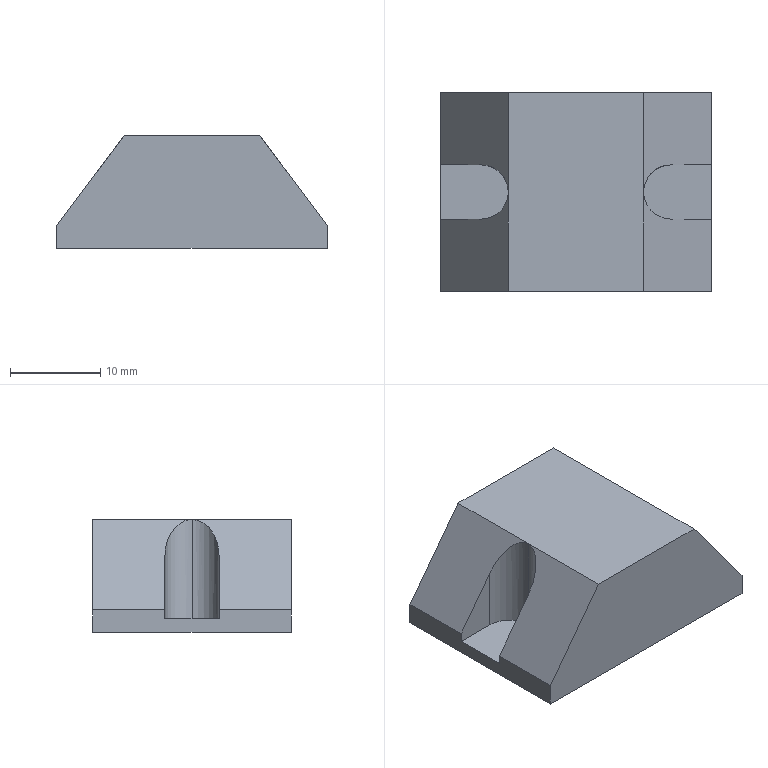Part | STEP file | Wire clamp block | 1 solid | 17 faces | box 30 x 22 x 12.5 mm | volume 6136 mm3 | plane 14 | cylinder 3 | commonest cylinder face diameters 6 x3
STEP:
#1=CARTESIAN_POINT('',(-7.5,0.,1.5));
#2=VERTEX_POINT('',#1);
#3=CARTESIAN_POINT('',(-10.5,3.,1.5));
#4=VERTEX_POINT('',#3);
#5=CARTESIAN_POINT('',(-10.5,0.,1.5));
#6=DIRECTION('',(0.,0.,1.));
#7=DIRECTION('',(1.,0.,0.));
#8=AXIS2_PLACEMENT_3D('',#5,#6,#7);
#9=CIRCLE('',#8,3.);
#10=EDGE_CURVE('',#2,#4,#9,.T.);
#11=ORIENTED_EDGE('',*,*,#10,.F.);
#12=CARTESIAN_POINT('',(-7.5,0.,12.486));
#13=VERTEX_POINT('',#12);
#14=CARTESIAN_POINT('',(-7.5,0.,1.5));
#15=DIRECTION('',(0.,0.,1.));
#16=VECTOR('',#15,1000.);
#17=LINE('',#14,#16);
#18=EDGE_CURVE('',#2,#13,#17,.T.);
#19=ORIENTED_EDGE('',*,*,#18,.T.);
#20=CARTESIAN_POINT('',(-10.5,3.,8.491));
#21=VERTEX_POINT('',#20);
#22=CARTESIAN_POINT('',(-7.5,0.,12.486));
#23=CARTESIAN_POINT('',(-7.5,1.757,12.486));
#24=CARTESIAN_POINT('',(-8.743,3.,10.831));
#25=CARTESIAN_POINT('',(-10.5,3.,8.491));
#26=(BOUNDED_CURVE()B_SPLINE_CURVE(3,(#22,#23,#24,#25),.UNSPECIFIED.,.F.,.T.)B_SPLINE_CURVE_WITH_KNOTS((4,4),(0.,1.571),.UNSPECIFIED.)CURVE()GEOMETRIC_REPRESENTATION_ITEM()RATIONAL_B_SPLINE_CURVE((1.,0.8047,0.8047,1.))REPRESENTATION_ITEM(''));
#27=EDGE_CURVE('',#13,#21,#26,.T.);
#28=ORIENTED_EDGE('',*,*,#27,.T.);
#29=CARTESIAN_POINT('',(-10.5,3.,1.5));
#30=DIRECTION('',(0.,0.,1.));
#31=VECTOR('',#30,1000.);
#32=LINE('',#29,#31);
#33=EDGE_CURVE('',#4,#21,#32,.T.);
#34=ORIENTED_EDGE('',*,*,#33,.F.);
#35=EDGE_LOOP('',(#11,#19,#28,#34));
#36=FACE_OUTER_BOUND('',#35,.T.);
#37=CARTESIAN_POINT('',(-10.5,0.,1.5));
#38=DIRECTION('',(0.,0.,1.));
#39=DIRECTION('',(1.,0.,0.));
#40=AXIS2_PLACEMENT_3D('',#37,#38,#39);
#41=CYLINDRICAL_SURFACE('',#40,3.);
#42=ADVANCED_FACE('',(#36),#41,.F.);
#43=CARTESIAN_POINT('',(-15.,-11.,0.));
#44=VERTEX_POINT('',#43);
#45=CARTESIAN_POINT('',(-15.,11.,0.));
#46=VERTEX_POINT('',#45);
#47=CARTESIAN_POINT('',(-15.,11.,0.));
#48=DIRECTION('',(0.,1.,0.));
#49=VECTOR('',#48,1000.);
#50=LINE('',#47,#49);
#51=EDGE_CURVE('',#44,#46,#50,.T.);
#52=ORIENTED_EDGE('',*,*,#51,.T.);
#53=CARTESIAN_POINT('',(15.,11.,0.));
#54=VERTEX_POINT('',#53);
#55=CARTESIAN_POINT('',(15.,11.,0.));
#56=DIRECTION('',(1.,0.,0.));
#57=VECTOR('',#56,1000.);
#58=LINE('',#55,#57);
#59=EDGE_CURVE('',#46,#54,#58,.T.);
#60=ORIENTED_EDGE('',*,*,#59,.T.);
#61=CARTESIAN_POINT('',(15.,-11.,0.));
#62=VERTEX_POINT('',#61);
#63=CARTESIAN_POINT('',(15.,11.,0.));
#64=DIRECTION('',(0.,-1.,0.));
#65=VECTOR('',#64,1000.);
#66=LINE('',#63,#65);
#67=EDGE_CURVE('',#54,#62,#66,.T.);
#68=ORIENTED_EDGE('',*,*,#67,.T.);
#69=CARTESIAN_POINT('',(15.,-11.,0.));
#70=DIRECTION('',(-1.,0.,0.));
#71=VECTOR('',#70,1000.);
#72=LINE('',#69,#71);
#73=EDGE_CURVE('',#62,#44,#72,.T.);
#74=ORIENTED_EDGE('',*,*,#73,.T.);
#75=EDGE_LOOP('',(#52,#60,#68,#74));
#76=FACE_OUTER_BOUND('',#75,.T.);
#77=CARTESIAN_POINT('',(15.,11.,0.));
#78=DIRECTION('',(0.,0.,-1.));
#79=DIRECTION('',(-1.,0.,0.));
#80=AXIS2_PLACEMENT_3D('',#77,#78,#79);
#81=PLANE('',#80);
#82=ADVANCED_FACE('',(#76),#81,.T.);
#83=CARTESIAN_POINT('',(-7.489,11.,12.5));
#84=VERTEX_POINT('',#83);
#85=CARTESIAN_POINT('',(-15.,11.,2.5));
#86=VERTEX_POINT('',#85);
#87=CARTESIAN_POINT('',(-7.489,11.,12.5));
#88=DIRECTION('',(-0.6006,0.,-0.7996));
#89=VECTOR('',#88,1000.);
#90=LINE('',#87,#89);
#91=EDGE_CURVE('',#84,#86,#90,.T.);
#92=ORIENTED_EDGE('',*,*,#91,.F.);
#93=CARTESIAN_POINT('',(7.489,11.,12.5));
#94=VERTEX_POINT('',#93);
#95=CARTESIAN_POINT('',(-15.,11.,12.5));
#96=DIRECTION('',(-1.,0.,0.));
#97=VECTOR('',#96,1000.);
#98=LINE('',#95,#97);
#99=EDGE_CURVE('',#94,#84,#98,.T.);
#100=ORIENTED_EDGE('',*,*,#99,.F.);
#101=CARTESIAN_POINT('',(15.,11.,2.5));
#102=VERTEX_POINT('',#101);
#103=CARTESIAN_POINT('',(15.,11.,2.5));
#104=DIRECTION('',(-0.6006,0.,0.7996));
#105=VECTOR('',#104,1000.);
#106=LINE('',#103,#105);
#107=EDGE_CURVE('',#102,#94,#106,.T.);
#108=ORIENTED_EDGE('',*,*,#107,.F.);
#109=CARTESIAN_POINT('',(15.,11.,12.5));
#110=DIRECTION('',(0.,0.,1.));
#111=VECTOR('',#110,1000.);
#112=LINE('',#109,#111);
#113=EDGE_CURVE('',#54,#102,#112,.T.);
#114=ORIENTED_EDGE('',*,*,#113,.F.);
#115=ORIENTED_EDGE('',*,*,#59,.F.);
#116=CARTESIAN_POINT('',(-15.,11.,12.5));
#117=DIRECTION('',(0.,0.,-1.));
#118=VECTOR('',#117,1000.);
#119=LINE('',#116,#118);
#120=EDGE_CURVE('',#86,#46,#119,.T.);
#121=ORIENTED_EDGE('',*,*,#120,.F.);
#122=EDGE_LOOP('',(#92,#100,#108,#114,#115,#121));
#123=FACE_OUTER_BOUND('',#122,.T.);
#124=CARTESIAN_POINT('',(-15.,11.,12.5));
#125=DIRECTION('',(0.,-1.,0.));
#126=DIRECTION('',(0.,0.,-1.));
#127=AXIS2_PLACEMENT_3D('',#124,#125,#126);
#128=PLANE('',#127);
#129=ADVANCED_FACE('',(#123),#128,.F.);
#130=CARTESIAN_POINT('',(-15.,-3.,2.5));
#131=VERTEX_POINT('',#130);
#132=CARTESIAN_POINT('',(-15.,-3.,1.5));
#133=VERTEX_POINT('',#132);
#134=CARTESIAN_POINT('',(-15.,-3.,1.5));
#135=DIRECTION('',(0.,0.,-1.));
#136=VECTOR('',#135,1000.);
#137=LINE('',#134,#136);
#138=EDGE_CURVE('',#131,#133,#137,.T.);
#139=ORIENTED_EDGE('',*,*,#138,.T.);
#140=CARTESIAN_POINT('',(-15.,3.,1.5));
#141=VERTEX_POINT('',#140);
#142=CARTESIAN_POINT('',(-15.,-11.,1.5));
#143=DIRECTION('',(0.,-1.,0.));
#144=VECTOR('',#143,1000.);
#145=LINE('',#142,#144);
#146=EDGE_CURVE('',#141,#133,#145,.T.);
#147=ORIENTED_EDGE('',*,*,#146,.F.);
#148=CARTESIAN_POINT('',(-15.,3.,2.5));
#149=VERTEX_POINT('',#148);
#150=CARTESIAN_POINT('',(-15.,3.,1.5));
#151=DIRECTION('',(0.,0.,1.));
#152=VECTOR('',#151,1000.);
#153=LINE('',#150,#152);
#154=EDGE_CURVE('',#141,#149,#153,.T.);
#155=ORIENTED_EDGE('',*,*,#154,.T.);
#156=CARTESIAN_POINT('',(-15.,-11.,2.5));
#157=DIRECTION('',(0.,-1.,0.));
#158=VECTOR('',#157,1000.);
#159=LINE('',#156,#158);
#160=EDGE_CURVE('',#86,#149,#159,.T.);
#161=ORIENTED_EDGE('',*,*,#160,.F.);
#162=ORIENTED_EDGE('',*,*,#120,.T.);
#163=ORIENTED_EDGE('',*,*,#51,.F.);
#164=CARTESIAN_POINT('',(-15.,-11.,2.5));
#165=VERTEX_POINT('',#164);
#166=CARTESIAN_POINT('',(-15.,-11.,12.5));
#167=DIRECTION('',(0.,0.,-1.));
#168=VECTOR('',#167,1000.);
#169=LINE('',#166,#168);
#170=EDGE_CURVE('',#165,#44,#169,.T.);
#171=ORIENTED_EDGE('',*,*,#170,.F.);
#172=CARTESIAN_POINT('',(-15.,-11.,2.5));
#173=DIRECTION('',(0.,-1.,0.));
#174=VECTOR('',#173,1000.);
#175=LINE('',#172,#174);
#176=EDGE_CURVE('',#131,#165,#175,.T.);
#177=ORIENTED_EDGE('',*,*,#176,.F.);
#178=EDGE_LOOP('',(#139,#147,#155,#161,#162,#163,#171,#177));
#179=FACE_OUTER_BOUND('',#178,.T.);
#180=CARTESIAN_POINT('',(-15.,-11.,12.5));
#181=DIRECTION('',(1.,0.,0.));
#182=DIRECTION('',(0.,0.,-1.));
#183=AXIS2_PLACEMENT_3D('',#180,#181,#182);
#184=PLANE('',#183);
#185=ADVANCED_FACE('',(#179),#184,.F.);
#186=CARTESIAN_POINT('',(-7.489,-11.,12.5));
#187=VERTEX_POINT('',#186);
#188=CARTESIAN_POINT('',(-15.,-11.,2.5));
#189=DIRECTION('',(0.6006,0.,0.7996));
#190=VECTOR('',#189,1000.);
#191=LINE('',#188,#190);
#192=EDGE_CURVE('',#165,#187,#191,.T.);
#193=ORIENTED_EDGE('',*,*,#192,.F.);
#194=ORIENTED_EDGE('',*,*,#170,.T.);
#195=ORIENTED_EDGE('',*,*,#73,.F.);
#196=CARTESIAN_POINT('',(15.,-11.,2.5));
#197=VERTEX_POINT('',#196);
#198=CARTESIAN_POINT('',(15.,-11.,12.5));
#199=DIRECTION('',(0.,0.,-1.));
#200=VECTOR('',#199,1000.);
#201=LINE('',#198,#200);
#202=EDGE_CURVE('',#197,#62,#201,.T.);
#203=ORIENTED_EDGE('',*,*,#202,.F.);
#204=CARTESIAN_POINT('',(7.489,-11.,12.5));
#205=VERTEX_POINT('',#204);
#206=CARTESIAN_POINT('',(7.489,-11.,12.5));
#207=DIRECTION('',(0.6006,0.,-0.7996));
#208=VECTOR('',#207,1000.);
#209=LINE('',#206,#208);
#210=EDGE_CURVE('',#205,#197,#209,.T.);
#211=ORIENTED_EDGE('',*,*,#210,.F.);
#212=CARTESIAN_POINT('',(-15.,-11.,12.5));
#213=DIRECTION('',(1.,0.,0.));
#214=VECTOR('',#213,1000.);
#215=LINE('',#212,#214);
#216=EDGE_CURVE('',#187,#205,#215,.T.);
#217=ORIENTED_EDGE('',*,*,#216,.F.);
#218=EDGE_LOOP('',(#193,#194,#195,#203,#211,#217));
#219=FACE_OUTER_BOUND('',#218,.T.);
#220=CARTESIAN_POINT('',(-15.,-11.,12.5));
#221=DIRECTION('',(0.,1.,0.));
#222=DIRECTION('',(0.,0.,1.));
#223=AXIS2_PLACEMENT_3D('',#220,#221,#222);
#224=PLANE('',#223);
#225=ADVANCED_FACE('',(#219),#224,.F.);
#226=CARTESIAN_POINT('',(15.,3.,2.5));
#227=VERTEX_POINT('',#226);
#228=CARTESIAN_POINT('',(15.,3.,1.5));
#229=VERTEX_POINT('',#228);
#230=CARTESIAN_POINT('',(15.,3.,1.5));
#231=DIRECTION('',(0.,0.,-1.));
#232=VECTOR('',#231,1000.);
#233=LINE('',#230,#232);
#234=EDGE_CURVE('',#227,#229,#233,.T.);
#235=ORIENTED_EDGE('',*,*,#234,.T.);
#236=CARTESIAN_POINT('',(15.,-3.,1.5));
#237=VERTEX_POINT('',#236);
#238=CARTESIAN_POINT('',(15.,-11.,1.5));
#239=DIRECTION('',(0.,1.,0.));
#240=VECTOR('',#239,1000.);
#241=LINE('',#238,#240);
#242=EDGE_CURVE('',#237,#229,#241,.T.);
#243=ORIENTED_EDGE('',*,*,#242,.F.);
#244=CARTESIAN_POINT('',(15.,-3.,2.5));
#245=VERTEX_POINT('',#244);
#246=CARTESIAN_POINT('',(15.,-3.,1.5));
#247=DIRECTION('',(0.,0.,1.));
#248=VECTOR('',#247,1000.);
#249=LINE('',#246,#248);
#250=EDGE_CURVE('',#237,#245,#249,.T.);
#251=ORIENTED_EDGE('',*,*,#250,.T.);
#252=CARTESIAN_POINT('',(15.,-11.,2.5));
#253=DIRECTION('',(0.,1.,0.));
#254=VECTOR('',#253,1000.);
#255=LINE('',#252,#254);
#256=EDGE_CURVE('',#197,#245,#255,.T.);
#257=ORIENTED_EDGE('',*,*,#256,.F.);
#258=ORIENTED_EDGE('',*,*,#202,.T.);
#259=ORIENTED_EDGE('',*,*,#67,.F.);
#260=ORIENTED_EDGE('',*,*,#113,.T.);
#261=CARTESIAN_POINT('',(15.,-11.,2.5));
#262=DIRECTION('',(0.,1.,0.));
#263=VECTOR('',#262,1000.);
#264=LINE('',#261,#263);
#265=EDGE_CURVE('',#227,#102,#264,.T.);
#266=ORIENTED_EDGE('',*,*,#265,.F.);
#267=EDGE_LOOP('',(#235,#243,#251,#257,#258,#259,#260,#266));
#268=FACE_OUTER_BOUND('',#267,.T.);
#269=CARTESIAN_POINT('',(15.,-11.,12.5));
#270=DIRECTION('',(-1.,0.,0.));
#271=DIRECTION('',(0.,0.,1.));
#272=AXIS2_PLACEMENT_3D('',#269,#270,#271);
#273=PLANE('',#272);
#274=ADVANCED_FACE('',(#268),#273,.F.);
#275=CARTESIAN_POINT('',(-10.5,-3.,8.491));
#276=VERTEX_POINT('',#275);
#277=CARTESIAN_POINT('',(-10.5,-3.,8.491));
#278=CARTESIAN_POINT('',(-8.743,-3.,10.831));
#279=CARTESIAN_POINT('',(-7.5,-1.757,12.486));
#280=CARTESIAN_POINT('',(-7.5,0.,12.486));
#281=(BOUNDED_CURVE()B_SPLINE_CURVE(3,(#277,#278,#279,#280),.UNSPECIFIED.,.F.,.F.)B_SPLINE_CURVE_WITH_KNOTS((4,4),(4.712,6.283),.UNSPECIFIED.)CURVE()GEOMETRIC_REPRESENTATION_ITEM()RATIONAL_B_SPLINE_CURVE((1.,0.8047,0.8047,1.))REPRESENTATION_ITEM(''));
#282=EDGE_CURVE('',#276,#13,#281,.T.);
#283=ORIENTED_EDGE('',*,*,#282,.F.);
#284=CARTESIAN_POINT('',(-15.,-3.,2.5));
#285=DIRECTION('',(0.6006,0.,0.7996));
#286=VECTOR('',#285,1000.);
#287=LINE('',#284,#286);
#288=EDGE_CURVE('',#131,#276,#287,.T.);
#289=ORIENTED_EDGE('',*,*,#288,.F.);
#290=ORIENTED_EDGE('',*,*,#176,.T.);
#291=ORIENTED_EDGE('',*,*,#192,.T.);
#292=CARTESIAN_POINT('',(-7.489,19.,12.5));
#293=DIRECTION('',(0.,-1.,0.));
#294=VECTOR('',#293,1000.);
#295=LINE('',#292,#294);
#296=EDGE_CURVE('',#84,#187,#295,.T.);
#297=ORIENTED_EDGE('',*,*,#296,.F.);
#298=ORIENTED_EDGE('',*,*,#91,.T.);
#299=ORIENTED_EDGE('',*,*,#160,.T.);
#300=CARTESIAN_POINT('',(-15.,3.,2.5));
#301=DIRECTION('',(-0.6006,0.,-0.7996));
#302=VECTOR('',#301,1000.);
#303=LINE('',#300,#302);
#304=EDGE_CURVE('',#21,#149,#303,.T.);
#305=ORIENTED_EDGE('',*,*,#304,.F.);
#306=ORIENTED_EDGE('',*,*,#27,.F.);
#307=EDGE_LOOP('',(#283,#289,#290,#291,#297,#298,#299,#305,#306));
#308=FACE_OUTER_BOUND('',#307,.T.);
#309=CARTESIAN_POINT('',(-15.,19.,2.5));
#310=DIRECTION('',(0.7996,0.,-0.6006));
#311=DIRECTION('',(-0.6006,0.,-0.7996));
#312=AXIS2_PLACEMENT_3D('',#309,#310,#311);
#313=PLANE('',#312);
#314=ADVANCED_FACE('',(#308),#313,.F.);
#315=ORIENTED_EDGE('',*,*,#296,.T.);
#316=ORIENTED_EDGE('',*,*,#216,.T.);
#317=CARTESIAN_POINT('',(7.489,11.,12.5));
#318=DIRECTION('',(0.,-1.,0.));
#319=VECTOR('',#318,1000.);
#320=LINE('',#317,#319);
#321=EDGE_CURVE('',#94,#205,#320,.T.);
#322=ORIENTED_EDGE('',*,*,#321,.F.);
#323=ORIENTED_EDGE('',*,*,#99,.T.);
#324=EDGE_LOOP('',(#315,#316,#322,#323));
#325=FACE_OUTER_BOUND('',#324,.T.);
#326=CARTESIAN_POINT('',(15.,11.,12.5));
#327=DIRECTION('',(0.,0.,-1.));
#328=DIRECTION('',(-1.,0.,0.));
#329=AXIS2_PLACEMENT_3D('',#326,#327,#328);
#330=PLANE('',#329);
#331=ADVANCED_FACE('',(#325),#330,.F.);
#332=CARTESIAN_POINT('',(10.5,3.,8.491));
#333=VERTEX_POINT('',#332);
#334=CARTESIAN_POINT('',(15.,3.,2.5));
#335=DIRECTION('',(-0.6006,0.,0.7996));
#336=VECTOR('',#335,1000.);
#337=LINE('',#334,#336);
#338=EDGE_CURVE('',#227,#333,#337,.T.);
#339=ORIENTED_EDGE('',*,*,#338,.F.);
#340=ORIENTED_EDGE('',*,*,#265,.T.);
#341=ORIENTED_EDGE('',*,*,#107,.T.);
#342=ORIENTED_EDGE('',*,*,#321,.T.);
#343=ORIENTED_EDGE('',*,*,#210,.T.);
#344=ORIENTED_EDGE('',*,*,#256,.T.);
#345=CARTESIAN_POINT('',(10.5,-3.,8.491));
#346=VERTEX_POINT('',#345);
#347=CARTESIAN_POINT('',(15.,-3.,2.5));
#348=DIRECTION('',(0.6006,0.,-0.7996));
#349=VECTOR('',#348,1000.);
#350=LINE('',#347,#349);
#351=EDGE_CURVE('',#346,#245,#350,.T.);
#352=ORIENTED_EDGE('',*,*,#351,.F.);
#353=CARTESIAN_POINT('',(10.5,3.,8.491));
#354=CARTESIAN_POINT('',(4.5,3.,16.48));
#355=CARTESIAN_POINT('',(4.5,-3.,16.48));
#356=CARTESIAN_POINT('',(10.5,-3.,8.491));
#357=(BOUNDED_CURVE()B_SPLINE_CURVE(3,(#353,#354,#355,#356),.UNSPECIFIED.,.F.,.F.)B_SPLINE_CURVE_WITH_KNOTS((4,4),(4.712,7.854),.UNSPECIFIED.)CURVE()GEOMETRIC_REPRESENTATION_ITEM()RATIONAL_B_SPLINE_CURVE((1.,0.3333,0.3333,1.))REPRESENTATION_ITEM(''));
#358=EDGE_CURVE('',#333,#346,#357,.T.);
#359=ORIENTED_EDGE('',*,*,#358,.F.);
#360=EDGE_LOOP('',(#339,#340,#341,#342,#343,#344,#352,#359));
#361=FACE_OUTER_BOUND('',#360,.T.);
#362=CARTESIAN_POINT('',(15.,19.,2.5));
#363=DIRECTION('',(-0.7996,0.,-0.6006));
#364=DIRECTION('',(-0.6006,0.,0.7996));
#365=AXIS2_PLACEMENT_3D('',#362,#363,#364);
#366=PLANE('',#365);
#367=ADVANCED_FACE('',(#361),#366,.F.);
#368=ORIENTED_EDGE('',*,*,#146,.T.);
#369=CARTESIAN_POINT('',(-10.5,-3.,1.5));
#370=VERTEX_POINT('',#369);
#371=CARTESIAN_POINT('',(-10.5,-3.,1.5));
#372=DIRECTION('',(1.,0.,0.));
#373=VECTOR('',#372,1000.);
#374=LINE('',#371,#373);
#375=EDGE_CURVE('',#133,#370,#374,.T.);
#376=ORIENTED_EDGE('',*,*,#375,.T.);
#377=CARTESIAN_POINT('',(-10.5,0.,1.5));
#378=DIRECTION('',(0.,0.,1.));
#379=DIRECTION('',(1.,0.,0.));
#380=AXIS2_PLACEMENT_3D('',#377,#378,#379);
#381=CIRCLE('',#380,3.);
#382=EDGE_CURVE('',#370,#2,#381,.T.);
#383=ORIENTED_EDGE('',*,*,#382,.T.);
#384=ORIENTED_EDGE('',*,*,#10,.T.);
#385=CARTESIAN_POINT('',(-10.5,3.,1.5));
#386=DIRECTION('',(-1.,0.,0.));
#387=VECTOR('',#386,1000.);
#388=LINE('',#385,#387);
#389=EDGE_CURVE('',#4,#141,#388,.T.);
#390=ORIENTED_EDGE('',*,*,#389,.T.);
#391=EDGE_LOOP('',(#368,#376,#383,#384,#390));
#392=FACE_OUTER_BOUND('',#391,.T.);
#393=CARTESIAN_POINT('',(-10.5,0.,1.5));
#394=DIRECTION('',(0.,0.,1.));
#395=DIRECTION('',(1.,0.,0.));
#396=AXIS2_PLACEMENT_3D('',#393,#394,#395);
#397=PLANE('',#396);
#398=ADVANCED_FACE('',(#392),#397,.T.);
#399=CARTESIAN_POINT('',(10.5,-3.,1.5));
#400=VERTEX_POINT('',#399);
#401=CARTESIAN_POINT('',(10.5,-3.,1.5));
#402=DIRECTION('',(-1.,0.,0.));
#403=VECTOR('',#402,1000.);
#404=LINE('',#401,#403);
#405=EDGE_CURVE('',#237,#400,#404,.T.);
#406=ORIENTED_EDGE('',*,*,#405,.F.);
#407=ORIENTED_EDGE('',*,*,#242,.T.);
#408=CARTESIAN_POINT('',(10.5,3.,1.5));
#409=VERTEX_POINT('',#408);
#410=CARTESIAN_POINT('',(10.5,3.,1.5));
#411=DIRECTION('',(1.,0.,0.));
#412=VECTOR('',#411,1000.);
#413=LINE('',#410,#412);
#414=EDGE_CURVE('',#409,#229,#413,.T.);
#415=ORIENTED_EDGE('',*,*,#414,.F.);
#416=CARTESIAN_POINT('',(10.5,0.,1.5));
#417=DIRECTION('',(0.,0.,-1.));
#418=DIRECTION('',(1.,0.,0.));
#419=AXIS2_PLACEMENT_3D('',#416,#417,#418);
#420=CIRCLE('',#419,3.);
#421=EDGE_CURVE('',#400,#409,#420,.T.);
#422=ORIENTED_EDGE('',*,*,#421,.F.);
#423=EDGE_LOOP('',(#406,#407,#415,#422));
#424=FACE_OUTER_BOUND('',#423,.T.);
#425=CARTESIAN_POINT('',(10.5,0.,1.5));
#426=DIRECTION('',(0.,0.,-1.));
#427=DIRECTION('',(-1.,0.,0.));
#428=AXIS2_PLACEMENT_3D('',#425,#426,#427);
#429=PLANE('',#428);
#430=ADVANCED_FACE('',(#424),#429,.F.);
#431=ORIENTED_EDGE('',*,*,#18,.F.);
#432=ORIENTED_EDGE('',*,*,#382,.F.);
#433=CARTESIAN_POINT('',(-10.5,-3.,1.5));
#434=DIRECTION('',(0.,0.,-1.));
#435=VECTOR('',#434,1000.);
#436=LINE('',#433,#435);
#437=EDGE_CURVE('',#276,#370,#436,.T.);
#438=ORIENTED_EDGE('',*,*,#437,.F.);
#439=ORIENTED_EDGE('',*,*,#282,.T.);
#440=EDGE_LOOP('',(#431,#432,#438,#439));
#441=FACE_OUTER_BOUND('',#440,.T.);
#442=CARTESIAN_POINT('',(-10.5,0.,1.5));
#443=DIRECTION('',(0.,0.,1.));
#444=DIRECTION('',(1.,0.,0.));
#445=AXIS2_PLACEMENT_3D('',#442,#443,#444);
#446=CYLINDRICAL_SURFACE('',#445,3.);
#447=ADVANCED_FACE('',(#441),#446,.F.);
#448=ORIENTED_EDGE('',*,*,#375,.F.);
#449=ORIENTED_EDGE('',*,*,#138,.F.);
#450=ORIENTED_EDGE('',*,*,#288,.T.);
#451=ORIENTED_EDGE('',*,*,#437,.T.);
#452=EDGE_LOOP('',(#448,#449,#450,#451));
#453=FACE_OUTER_BOUND('',#452,.T.);
#454=CARTESIAN_POINT('',(-10.5,-3.,1.5));
#455=DIRECTION('',(0.,-1.,0.));
#456=DIRECTION('',(0.,0.,-1.));
#457=AXIS2_PLACEMENT_3D('',#454,#455,#456);
#458=PLANE('',#457);
#459=ADVANCED_FACE('',(#453),#458,.F.);
#460=ORIENTED_EDGE('',*,*,#389,.F.);
#461=ORIENTED_EDGE('',*,*,#33,.T.);
#462=ORIENTED_EDGE('',*,*,#304,.T.);
#463=ORIENTED_EDGE('',*,*,#154,.F.);
#464=EDGE_LOOP('',(#460,#461,#462,#463));
#465=FACE_OUTER_BOUND('',#464,.T.);
#466=CARTESIAN_POINT('',(-10.5,3.,1.5));
#467=DIRECTION('',(0.,1.,0.));
#468=DIRECTION('',(0.,0.,1.));
#469=AXIS2_PLACEMENT_3D('',#466,#467,#468);
#470=PLANE('',#469);
#471=ADVANCED_FACE('',(#465),#470,.F.);
#472=ORIENTED_EDGE('',*,*,#421,.T.);
#473=CARTESIAN_POINT('',(10.5,3.,1.5));
#474=DIRECTION('',(0.,0.,-1.));
#475=VECTOR('',#474,1000.);
#476=LINE('',#473,#475);
#477=EDGE_CURVE('',#333,#409,#476,.T.);
#478=ORIENTED_EDGE('',*,*,#477,.F.);
#479=ORIENTED_EDGE('',*,*,#358,.T.);
#480=CARTESIAN_POINT('',(10.5,-3.,1.5));
#481=DIRECTION('',(0.,0.,1.));
#482=VECTOR('',#481,1000.);
#483=LINE('',#480,#482);
#484=EDGE_CURVE('',#400,#346,#483,.T.);
#485=ORIENTED_EDGE('',*,*,#484,.F.);
#486=EDGE_LOOP('',(#472,#478,#479,#485));
#487=FACE_OUTER_BOUND('',#486,.T.);
#488=CARTESIAN_POINT('',(10.5,0.,1.5));
#489=DIRECTION('',(0.,0.,1.));
#490=DIRECTION('',(1.,0.,0.));
#491=AXIS2_PLACEMENT_3D('',#488,#489,#490);
#492=CYLINDRICAL_SURFACE('',#491,3.);
#493=ADVANCED_FACE('',(#487),#492,.F.);
#494=ORIENTED_EDGE('',*,*,#414,.T.);
#495=ORIENTED_EDGE('',*,*,#234,.F.);
#496=ORIENTED_EDGE('',*,*,#338,.T.);
#497=ORIENTED_EDGE('',*,*,#477,.T.);
#498=EDGE_LOOP('',(#494,#495,#496,#497));
#499=FACE_OUTER_BOUND('',#498,.T.);
#500=CARTESIAN_POINT('',(10.5,3.,1.5));
#501=DIRECTION('',(0.,1.,0.));
#502=DIRECTION('',(0.,0.,1.));
#503=AXIS2_PLACEMENT_3D('',#500,#501,#502);
#504=PLANE('',#503);
#505=ADVANCED_FACE('',(#499),#504,.F.);
#506=ORIENTED_EDGE('',*,*,#405,.T.);
#507=ORIENTED_EDGE('',*,*,#484,.T.);
#508=ORIENTED_EDGE('',*,*,#351,.T.);
#509=ORIENTED_EDGE('',*,*,#250,.F.);
#510=EDGE_LOOP('',(#506,#507,#508,#509));
#511=FACE_OUTER_BOUND('',#510,.T.);
#512=CARTESIAN_POINT('',(10.5,-3.,1.5));
#513=DIRECTION('',(0.,-1.,0.));
#514=DIRECTION('',(0.,0.,-1.));
#515=AXIS2_PLACEMENT_3D('',#512,#513,#514);
#516=PLANE('',#515);
#517=ADVANCED_FACE('',(#511),#516,.F.);
#518=CLOSED_SHELL('',(#42,#82,#129,#185,#225,#274,#314,#331,#367,#398,#430,#447,#459,#471,#493,#505,#517));
#519=MANIFOLD_SOLID_BREP('',#518);
#520=CARTESIAN_POINT('',(0.,0.,0.));
#521=DIRECTION('',(0.,0.,1.));
#522=DIRECTION('',(1.,0.,0.));
#523=AXIS2_PLACEMENT_3D('',#520,#521,#522);
#524=(LENGTH_UNIT()NAMED_UNIT(*)SI_UNIT(.MILLI.,.METRE.));
#525=UNCERTAINTY_MEASURE_WITH_UNIT(LENGTH_MEASURE(0.00001),#524,'','');
#526=(NAMED_UNIT(*)PLANE_ANGLE_UNIT()SI_UNIT($,.RADIAN.));
#527=(NAMED_UNIT(*)SI_UNIT($,.STERADIAN.)SOLID_ANGLE_UNIT());
#528=(GEOMETRIC_REPRESENTATION_CONTEXT(3)GLOBAL_UNCERTAINTY_ASSIGNED_CONTEXT((#525))GLOBAL_UNIT_ASSIGNED_CONTEXT((#524,#526,#527))REPRESENTATION_CONTEXT('',''));
#529=ADVANCED_BREP_SHAPE_REPRESENTATION('',(#519,#523),#528);